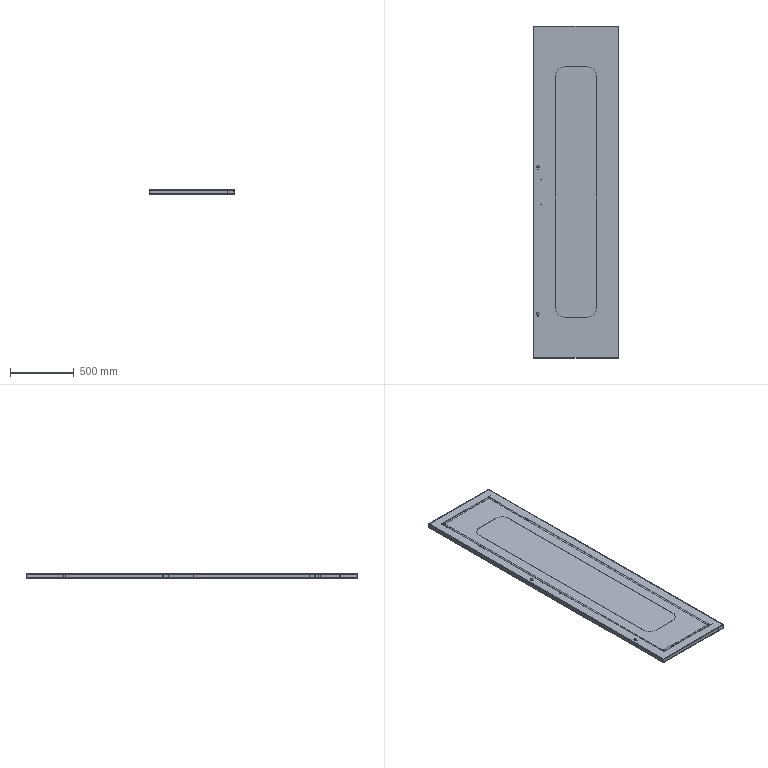Part | SolidWorks | features MirrorCompFeat 6, ReferencePattern 4, AEMSimFeature 1 | 10 solids | 598 faces | box 666 x 2594 x 35 mm | volume 4997012 mm3 | cylinder 348 | plane 234 | spline 16 | commonest cylinder face diameters 4 x108 3 x106 5.5 x20 10 x18 20 x16 2.4 x12